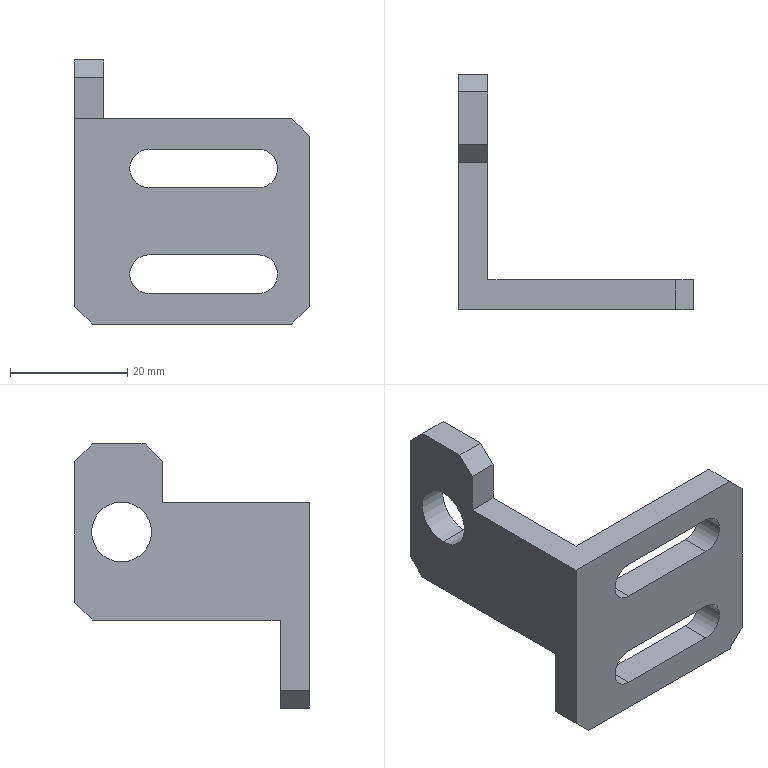Part | SolidWorks | features HoleWzd 2, ICE 2, Chamfer 1, Extrusion 1 | 1 solid | 27 faces | box 40 x 40 x 45 mm | volume 9137 mm3 | plane 21 | cylinder 6 | commonest cylinder face diameters 6.6 x4 10.2 x2
STEP:
#1=CARTESIAN_POINT('',(0.,-8.,35.1));
#2=VERTEX_POINT('',#1);
#3=CARTESIAN_POINT('',(0.,-8.,24.9));
#4=VERTEX_POINT('',#3);
#5=CARTESIAN_POINT('',(0.,-8.,30.));
#6=DIRECTION('',(1.,0.,0.));
#7=DIRECTION('',(0.,0.,-1.));
#8=AXIS2_PLACEMENT_3D('',#5,#6,#7);
#9=CIRCLE('',#8,5.1);
#10=EDGE_CURVE('',#2,#4,#9,.T.);
#11=ORIENTED_EDGE('',*,*,#10,.F.);
#12=CARTESIAN_POINT('',(5.,-8.,35.1));
#13=VERTEX_POINT('',#12);
#14=CARTESIAN_POINT('',(5.,-8.,35.1));
#15=DIRECTION('',(1.,0.,0.));
#16=VECTOR('',#15,1000.);
#17=LINE('',#14,#16);
#18=EDGE_CURVE('',#2,#13,#17,.T.);
#19=ORIENTED_EDGE('',*,*,#18,.T.);
#20=CARTESIAN_POINT('',(5.,-8.,24.9));
#21=VERTEX_POINT('',#20);
#22=CARTESIAN_POINT('',(5.,-8.,30.));
#23=DIRECTION('',(1.,0.,0.));
#24=DIRECTION('',(0.,0.,-1.));
#25=AXIS2_PLACEMENT_3D('',#22,#23,#24);
#26=CIRCLE('',#25,5.1);
#27=EDGE_CURVE('',#13,#21,#26,.T.);
#28=ORIENTED_EDGE('',*,*,#27,.T.);
#29=CARTESIAN_POINT('',(5.,-8.,24.9));
#30=DIRECTION('',(1.,0.,0.));
#31=VECTOR('',#30,1000.);
#32=LINE('',#29,#31);
#33=EDGE_CURVE('',#4,#21,#32,.T.);
#34=ORIENTED_EDGE('',*,*,#33,.F.);
#35=EDGE_LOOP('',(#11,#19,#28,#34));
#36=FACE_OUTER_BOUND('',#35,.T.);
#37=CARTESIAN_POINT('',(5.,-8.,30.));
#38=DIRECTION('',(1.,0.,0.));
#39=DIRECTION('',(0.,0.,-1.));
#40=AXIS2_PLACEMENT_3D('',#37,#38,#39);
#41=CYLINDRICAL_SURFACE('',#40,5.1);
#42=ADVANCED_FACE('',(#36),#41,.F.);
#43=CARTESIAN_POINT('',(12.7,-35.,5.2));
#44=VERTEX_POINT('',#43);
#45=CARTESIAN_POINT('',(12.7,-35.,11.8));
#46=VERTEX_POINT('',#45);
#47=CARTESIAN_POINT('',(12.7,-35.,8.5));
#48=DIRECTION('',(0.,1.,0.));
#49=DIRECTION('',(0.,0.,1.));
#50=AXIS2_PLACEMENT_3D('',#47,#48,#49);
#51=CIRCLE('',#50,3.3);
#52=EDGE_CURVE('',#44,#46,#51,.T.);
#53=ORIENTED_EDGE('',*,*,#52,.F.);
#54=CARTESIAN_POINT('',(31.3,-35.,5.2));
#55=VERTEX_POINT('',#54);
#56=CARTESIAN_POINT('',(12.7,-35.,5.2));
#57=DIRECTION('',(1.,0.,0.));
#58=VECTOR('',#57,1000.);
#59=LINE('',#56,#58);
#60=EDGE_CURVE('',#44,#55,#59,.T.);
#61=ORIENTED_EDGE('',*,*,#60,.T.);
#62=CARTESIAN_POINT('',(31.3,-35.,11.8));
#63=VERTEX_POINT('',#62);
#64=CARTESIAN_POINT('',(31.3,-35.,8.5));
#65=DIRECTION('',(0.,1.,0.));
#66=DIRECTION('',(0.,0.,1.));
#67=AXIS2_PLACEMENT_3D('',#64,#65,#66);
#68=CIRCLE('',#67,3.3);
#69=EDGE_CURVE('',#63,#55,#68,.T.);
#70=ORIENTED_EDGE('',*,*,#69,.F.);
#71=CARTESIAN_POINT('',(12.7,-35.,11.8));
#72=DIRECTION('',(1.,0.,0.));
#73=VECTOR('',#72,1000.);
#74=LINE('',#71,#73);
#75=EDGE_CURVE('',#46,#63,#74,.T.);
#76=ORIENTED_EDGE('',*,*,#75,.F.);
#77=EDGE_LOOP('',(#53,#61,#70,#76));
#78=FACE_BOUND('',#77,.T.);
#79=CARTESIAN_POINT('',(5.,-35.,35.));
#80=VERTEX_POINT('',#79);
#81=CARTESIAN_POINT('',(37.,-35.,35.));
#82=VERTEX_POINT('',#81);
#83=CARTESIAN_POINT('',(5.,-35.,35.));
#84=DIRECTION('',(1.,0.,0.));
#85=VECTOR('',#84,1000.);
#86=LINE('',#83,#85);
#87=EDGE_CURVE('',#80,#82,#86,.T.);
#88=ORIENTED_EDGE('',*,*,#87,.T.);
#89=CARTESIAN_POINT('',(40.,-35.,32.));
#90=VERTEX_POINT('',#89);
#91=CARTESIAN_POINT('',(40.,-35.,32.));
#92=DIRECTION('',(0.7071,0.,-0.7071));
#93=VECTOR('',#92,1000.);
#94=LINE('',#91,#93);
#95=EDGE_CURVE('',#82,#90,#94,.T.);
#96=ORIENTED_EDGE('',*,*,#95,.T.);
#97=CARTESIAN_POINT('',(40.,-35.,3.));
#98=VERTEX_POINT('',#97);
#99=CARTESIAN_POINT('',(40.,-35.,45.));
#100=DIRECTION('',(0.,0.,-1.));
#101=VECTOR('',#100,1000.);
#102=LINE('',#99,#101);
#103=EDGE_CURVE('',#90,#98,#102,.T.);
#104=ORIENTED_EDGE('',*,*,#103,.T.);
#105=CARTESIAN_POINT('',(37.,-35.,0.));
#106=VERTEX_POINT('',#105);
#107=CARTESIAN_POINT('',(40.,-35.,3.));
#108=DIRECTION('',(-0.7071,0.,-0.7071));
#109=VECTOR('',#108,1000.);
#110=LINE('',#107,#109);
#111=EDGE_CURVE('',#98,#106,#110,.T.);
#112=ORIENTED_EDGE('',*,*,#111,.T.);
#113=CARTESIAN_POINT('',(3.,-35.,0.));
#114=VERTEX_POINT('',#113);
#115=CARTESIAN_POINT('',(5.,-35.,0.));
#116=DIRECTION('',(-1.,0.,0.));
#117=VECTOR('',#116,1000.);
#118=LINE('',#115,#117);
#119=EDGE_CURVE('',#106,#114,#118,.T.);
#120=ORIENTED_EDGE('',*,*,#119,.T.);
#121=CARTESIAN_POINT('',(0.,-35.,3.));
#122=VERTEX_POINT('',#121);
#123=CARTESIAN_POINT('',(0.,-35.,3.));
#124=DIRECTION('',(-0.7071,0.,0.7071));
#125=VECTOR('',#124,1000.);
#126=LINE('',#123,#125);
#127=EDGE_CURVE('',#114,#122,#126,.T.);
#128=ORIENTED_EDGE('',*,*,#127,.T.);
#129=CARTESIAN_POINT('',(0.,-35.,15.));
#130=VERTEX_POINT('',#129);
#131=CARTESIAN_POINT('',(0.,-35.,0.));
#132=DIRECTION('',(0.,0.,1.));
#133=VECTOR('',#132,1000.);
#134=LINE('',#131,#133);
#135=EDGE_CURVE('',#122,#130,#134,.T.);
#136=ORIENTED_EDGE('',*,*,#135,.T.);
#137=CARTESIAN_POINT('',(5.,-35.,15.));
#138=VERTEX_POINT('',#137);
#139=CARTESIAN_POINT('',(5.,-35.,15.));
#140=DIRECTION('',(-1.,0.,0.));
#141=VECTOR('',#140,1000.);
#142=LINE('',#139,#141);
#143=EDGE_CURVE('',#138,#130,#142,.T.);
#144=ORIENTED_EDGE('',*,*,#143,.F.);
#145=CARTESIAN_POINT('',(5.,-35.,45.));
#146=DIRECTION('',(0.,0.,-1.));
#147=VECTOR('',#146,1000.);
#148=LINE('',#145,#147);
#149=EDGE_CURVE('',#80,#138,#148,.T.);
#150=ORIENTED_EDGE('',*,*,#149,.F.);
#151=EDGE_LOOP('',(#88,#96,#104,#112,#120,#128,#136,#144,#150));
#152=FACE_OUTER_BOUND('',#151,.T.);
#153=CARTESIAN_POINT('',(31.3,-35.,29.8));
#154=VERTEX_POINT('',#153);
#155=CARTESIAN_POINT('',(31.3,-35.,23.2));
#156=VERTEX_POINT('',#155);
#157=CARTESIAN_POINT('',(31.3,-35.,26.5));
#158=DIRECTION('',(0.,1.,0.));
#159=DIRECTION('',(0.,0.,1.));
#160=AXIS2_PLACEMENT_3D('',#157,#158,#159);
#161=CIRCLE('',#160,3.3);
#162=EDGE_CURVE('',#154,#156,#161,.T.);
#163=ORIENTED_EDGE('',*,*,#162,.F.);
#164=CARTESIAN_POINT('',(12.7,-35.,29.8));
#165=VERTEX_POINT('',#164);
#166=CARTESIAN_POINT('',(12.7,-35.,29.8));
#167=DIRECTION('',(1.,0.,0.));
#168=VECTOR('',#167,1000.);
#169=LINE('',#166,#168);
#170=EDGE_CURVE('',#165,#154,#169,.T.);
#171=ORIENTED_EDGE('',*,*,#170,.F.);
#172=CARTESIAN_POINT('',(12.7,-35.,23.2));
#173=VERTEX_POINT('',#172);
#174=CARTESIAN_POINT('',(12.7,-35.,26.5));
#175=DIRECTION('',(0.,1.,0.));
#176=DIRECTION('',(0.,0.,1.));
#177=AXIS2_PLACEMENT_3D('',#174,#175,#176);
#178=CIRCLE('',#177,3.3);
#179=EDGE_CURVE('',#173,#165,#178,.T.);
#180=ORIENTED_EDGE('',*,*,#179,.F.);
#181=CARTESIAN_POINT('',(12.7,-35.,23.2));
#182=DIRECTION('',(1.,0.,0.));
#183=VECTOR('',#182,1000.);
#184=LINE('',#181,#183);
#185=EDGE_CURVE('',#173,#156,#184,.T.);
#186=ORIENTED_EDGE('',*,*,#185,.T.);
#187=EDGE_LOOP('',(#163,#171,#180,#186));
#188=FACE_BOUND('',#187,.T.);
#189=CARTESIAN_POINT('',(5.,-35.,45.));
#190=DIRECTION('',(0.,-1.,0.));
#191=DIRECTION('',(0.,0.,-1.));
#192=AXIS2_PLACEMENT_3D('',#189,#190,#191);
#193=PLANE('',#192);
#194=ADVANCED_FACE('',(#78,#152,#188),#193,.F.);
#195=CARTESIAN_POINT('',(0.,-8.,30.));
#196=DIRECTION('',(1.,0.,0.));
#197=DIRECTION('',(0.,0.,-1.));
#198=AXIS2_PLACEMENT_3D('',#195,#196,#197);
#199=CIRCLE('',#198,5.1);
#200=EDGE_CURVE('',#4,#2,#199,.T.);
#201=ORIENTED_EDGE('',*,*,#200,.T.);
#202=ORIENTED_EDGE('',*,*,#10,.T.);
#203=EDGE_LOOP('',(#201,#202));
#204=FACE_BOUND('',#203,.T.);
#205=ORIENTED_EDGE('',*,*,#135,.F.);
#206=CARTESIAN_POINT('',(0.,-40.,3.));
#207=VERTEX_POINT('',#206);
#208=CARTESIAN_POINT('',(0.,-40.,3.));
#209=DIRECTION('',(0.,-1.,0.));
#210=VECTOR('',#209,1000.);
#211=LINE('',#208,#210);
#212=EDGE_CURVE('',#122,#207,#211,.T.);
#213=ORIENTED_EDGE('',*,*,#212,.T.);
#214=CARTESIAN_POINT('',(0.,-40.,35.));
#215=VERTEX_POINT('',#214);
#216=CARTESIAN_POINT('',(0.,-40.,45.));
#217=DIRECTION('',(0.,0.,-1.));
#218=VECTOR('',#217,1000.);
#219=LINE('',#216,#218);
#220=EDGE_CURVE('',#215,#207,#219,.T.);
#221=ORIENTED_EDGE('',*,*,#220,.F.);
#222=CARTESIAN_POINT('',(0.,-15.,35.));
#223=VERTEX_POINT('',#222);
#224=CARTESIAN_POINT('',(0.,-40.,35.));
#225=DIRECTION('',(0.,-1.,0.));
#226=VECTOR('',#225,1000.);
#227=LINE('',#224,#226);
#228=EDGE_CURVE('',#223,#215,#227,.T.);
#229=ORIENTED_EDGE('',*,*,#228,.F.);
#230=CARTESIAN_POINT('',(0.,-15.,42.));
#231=VERTEX_POINT('',#230);
#232=CARTESIAN_POINT('',(0.,-15.,45.));
#233=DIRECTION('',(0.,0.,-1.));
#234=VECTOR('',#233,1000.);
#235=LINE('',#232,#234);
#236=EDGE_CURVE('',#231,#223,#235,.T.);
#237=ORIENTED_EDGE('',*,*,#236,.F.);
#238=CARTESIAN_POINT('',(0.,-12.,45.));
#239=VERTEX_POINT('',#238);
#240=CARTESIAN_POINT('',(0.,-15.,42.));
#241=DIRECTION('',(0.,0.7071,0.7071));
#242=VECTOR('',#241,1000.);
#243=LINE('',#240,#242);
#244=EDGE_CURVE('',#231,#239,#243,.T.);
#245=ORIENTED_EDGE('',*,*,#244,.T.);
#246=CARTESIAN_POINT('',(0.,-3.,45.));
#247=VERTEX_POINT('',#246);
#248=CARTESIAN_POINT('',(0.,-40.,45.));
#249=DIRECTION('',(0.,-1.,0.));
#250=VECTOR('',#249,1000.);
#251=LINE('',#248,#250);
#252=EDGE_CURVE('',#247,#239,#251,.T.);
#253=ORIENTED_EDGE('',*,*,#252,.F.);
#254=CARTESIAN_POINT('',(0.,0.,42.));
#255=VERTEX_POINT('',#254);
#256=CARTESIAN_POINT('',(0.,-3.,45.));
#257=DIRECTION('',(0.,0.7071,-0.7071));
#258=VECTOR('',#257,1000.);
#259=LINE('',#256,#258);
#260=EDGE_CURVE('',#247,#255,#259,.T.);
#261=ORIENTED_EDGE('',*,*,#260,.T.);
#262=CARTESIAN_POINT('',(0.,0.,18.));
#263=VERTEX_POINT('',#262);
#264=CARTESIAN_POINT('',(0.,0.,45.));
#265=DIRECTION('',(0.,0.,-1.));
#266=VECTOR('',#265,1000.);
#267=LINE('',#264,#266);
#268=EDGE_CURVE('',#255,#263,#267,.T.);
#269=ORIENTED_EDGE('',*,*,#268,.T.);
#270=CARTESIAN_POINT('',(0.,-3.,15.));
#271=VERTEX_POINT('',#270);
#272=CARTESIAN_POINT('',(0.,0.,18.));
#273=DIRECTION('',(0.,-0.7071,-0.7071));
#274=VECTOR('',#273,1000.);
#275=LINE('',#272,#274);
#276=EDGE_CURVE('',#263,#271,#275,.T.);
#277=ORIENTED_EDGE('',*,*,#276,.T.);
#278=CARTESIAN_POINT('',(0.,0.,15.));
#279=DIRECTION('',(0.,1.,0.));
#280=VECTOR('',#279,1000.);
#281=LINE('',#278,#280);
#282=EDGE_CURVE('',#130,#271,#281,.T.);
#283=ORIENTED_EDGE('',*,*,#282,.F.);
#284=EDGE_LOOP('',(#205,#213,#221,#229,#237,#245,#253,#261,#269,#277,#283));
#285=FACE_OUTER_BOUND('',#284,.T.);
#286=CARTESIAN_POINT('',(0.,-40.,45.));
#287=DIRECTION('',(1.,0.,0.));
#288=DIRECTION('',(0.,0.,-1.));
#289=AXIS2_PLACEMENT_3D('',#286,#287,#288);
#290=PLANE('',#289);
#291=ADVANCED_FACE('',(#204,#285),#290,.F.);
#292=CARTESIAN_POINT('',(31.3,-40.,11.8));
#293=VERTEX_POINT('',#292);
#294=CARTESIAN_POINT('',(31.3,-40.,5.2));
#295=VERTEX_POINT('',#294);
#296=CARTESIAN_POINT('',(31.3,-40.,8.5));
#297=DIRECTION('',(0.,1.,0.));
#298=DIRECTION('',(-1.,0.,0.));
#299=AXIS2_PLACEMENT_3D('',#296,#297,#298);
#300=CIRCLE('',#299,3.3);
#301=EDGE_CURVE('',#293,#295,#300,.T.);
#302=ORIENTED_EDGE('',*,*,#301,.T.);
#303=CARTESIAN_POINT('',(12.7,-40.,5.2));
#304=VERTEX_POINT('',#303);
#305=CARTESIAN_POINT('',(40.,-40.,5.2));
#306=DIRECTION('',(-1.,0.,0.));
#307=VECTOR('',#306,1000.);
#308=LINE('',#305,#307);
#309=EDGE_CURVE('',#295,#304,#308,.T.);
#310=ORIENTED_EDGE('',*,*,#309,.T.);
#311=CARTESIAN_POINT('',(12.7,-40.,11.8));
#312=VERTEX_POINT('',#311);
#313=CARTESIAN_POINT('',(12.7,-40.,8.5));
#314=DIRECTION('',(0.,1.,0.));
#315=DIRECTION('',(-1.,0.,0.));
#316=AXIS2_PLACEMENT_3D('',#313,#314,#315);
#317=CIRCLE('',#316,3.3);
#318=EDGE_CURVE('',#304,#312,#317,.T.);
#319=ORIENTED_EDGE('',*,*,#318,.T.);
#320=CARTESIAN_POINT('',(40.,-40.,11.8));
#321=DIRECTION('',(1.,0.,0.));
#322=VECTOR('',#321,1000.);
#323=LINE('',#320,#322);
#324=EDGE_CURVE('',#312,#293,#323,.T.);
#325=ORIENTED_EDGE('',*,*,#324,.T.);
#326=EDGE_LOOP('',(#302,#310,#319,#325));
#327=FACE_BOUND('',#326,.T.);
#328=CARTESIAN_POINT('',(12.7,-40.,29.8));
#329=VERTEX_POINT('',#328);
#330=CARTESIAN_POINT('',(31.3,-40.,29.8));
#331=VERTEX_POINT('',#330);
#332=CARTESIAN_POINT('',(40.,-40.,29.8));
#333=DIRECTION('',(1.,0.,0.));
#334=VECTOR('',#333,1000.);
#335=LINE('',#332,#334);
#336=EDGE_CURVE('',#329,#331,#335,.T.);
#337=ORIENTED_EDGE('',*,*,#336,.T.);
#338=CARTESIAN_POINT('',(31.3,-40.,23.2));
#339=VERTEX_POINT('',#338);
#340=CARTESIAN_POINT('',(31.3,-40.,26.5));
#341=DIRECTION('',(0.,1.,0.));
#342=DIRECTION('',(-1.,0.,0.));
#343=AXIS2_PLACEMENT_3D('',#340,#341,#342);
#344=CIRCLE('',#343,3.3);
#345=EDGE_CURVE('',#331,#339,#344,.T.);
#346=ORIENTED_EDGE('',*,*,#345,.T.);
#347=CARTESIAN_POINT('',(12.7,-40.,23.2));
#348=VERTEX_POINT('',#347);
#349=CARTESIAN_POINT('',(40.,-40.,23.2));
#350=DIRECTION('',(-1.,0.,0.));
#351=VECTOR('',#350,1000.);
#352=LINE('',#349,#351);
#353=EDGE_CURVE('',#339,#348,#352,.T.);
#354=ORIENTED_EDGE('',*,*,#353,.T.);
#355=CARTESIAN_POINT('',(12.7,-40.,26.5));
#356=DIRECTION('',(0.,1.,0.));
#357=DIRECTION('',(-1.,0.,0.));
#358=AXIS2_PLACEMENT_3D('',#355,#356,#357);
#359=CIRCLE('',#358,3.3);
#360=EDGE_CURVE('',#348,#329,#359,.T.);
#361=ORIENTED_EDGE('',*,*,#360,.T.);
#362=EDGE_LOOP('',(#337,#346,#354,#361));
#363=FACE_BOUND('',#362,.T.);
#364=CARTESIAN_POINT('',(40.,-40.,32.));
#365=VERTEX_POINT('',#364);
#366=CARTESIAN_POINT('',(40.,-40.,3.));
#367=VERTEX_POINT('',#366);
#368=CARTESIAN_POINT('',(40.,-40.,45.));
#369=DIRECTION('',(0.,0.,-1.));
#370=VECTOR('',#369,1000.);
#371=LINE('',#368,#370);
#372=EDGE_CURVE('',#365,#367,#371,.T.);
#373=ORIENTED_EDGE('',*,*,#372,.F.);
#374=CARTESIAN_POINT('',(37.,-40.,35.));
#375=VERTEX_POINT('',#374);
#376=CARTESIAN_POINT('',(40.,-40.,32.));
#377=DIRECTION('',(-0.7071,0.,0.7071));
#378=VECTOR('',#377,1000.);
#379=LINE('',#376,#378);
#380=EDGE_CURVE('',#365,#375,#379,.T.);
#381=ORIENTED_EDGE('',*,*,#380,.T.);
#382=CARTESIAN_POINT('',(5.,-40.,35.));
#383=DIRECTION('',(-1.,0.,0.));
#384=VECTOR('',#383,1000.);
#385=LINE('',#382,#384);
#386=EDGE_CURVE('',#375,#215,#385,.T.);
#387=ORIENTED_EDGE('',*,*,#386,.T.);
#388=ORIENTED_EDGE('',*,*,#220,.T.);
#389=CARTESIAN_POINT('',(3.,-40.,0.));
#390=VERTEX_POINT('',#389);
#391=CARTESIAN_POINT('',(0.,-40.,3.));
#392=DIRECTION('',(0.7071,0.,-0.7071));
#393=VECTOR('',#392,1000.);
#394=LINE('',#391,#393);
#395=EDGE_CURVE('',#207,#390,#394,.T.);
#396=ORIENTED_EDGE('',*,*,#395,.T.);
#397=CARTESIAN_POINT('',(37.,-40.,0.));
#398=VERTEX_POINT('',#397);
#399=CARTESIAN_POINT('',(40.,-40.,0.));
#400=DIRECTION('',(1.,0.,0.));
#401=VECTOR('',#400,1000.);
#402=LINE('',#399,#401);
#403=EDGE_CURVE('',#390,#398,#402,.T.);
#404=ORIENTED_EDGE('',*,*,#403,.T.);
#405=CARTESIAN_POINT('',(40.,-40.,3.));
#406=DIRECTION('',(0.7071,0.,0.7071));
#407=VECTOR('',#406,1000.);
#408=LINE('',#405,#407);
#409=EDGE_CURVE('',#398,#367,#408,.T.);
#410=ORIENTED_EDGE('',*,*,#409,.T.);
#411=EDGE_LOOP('',(#373,#381,#387,#388,#396,#404,#410));
#412=FACE_OUTER_BOUND('',#411,.T.);
#413=CARTESIAN_POINT('',(40.,-40.,45.));
#414=DIRECTION('',(0.,1.,0.));
#415=DIRECTION('',(-1.,0.,0.));
#416=AXIS2_PLACEMENT_3D('',#413,#414,#415);
#417=PLANE('',#416);
#418=ADVANCED_FACE('',(#327,#363,#412),#417,.F.);
#419=ORIENTED_EDGE('',*,*,#103,.F.);
#420=CARTESIAN_POINT('',(40.,-35.,32.));
#421=DIRECTION('',(0.,-1.,0.));
#422=VECTOR('',#421,1000.);
#423=LINE('',#420,#422);
#424=EDGE_CURVE('',#90,#365,#423,.T.);
#425=ORIENTED_EDGE('',*,*,#424,.T.);
#426=ORIENTED_EDGE('',*,*,#372,.T.);
#427=CARTESIAN_POINT('',(40.,-35.,3.));
#428=DIRECTION('',(0.,1.,0.));
#429=VECTOR('',#428,1000.);
#430=LINE('',#427,#429);
#431=EDGE_CURVE('',#367,#98,#430,.T.);
#432=ORIENTED_EDGE('',*,*,#431,.T.);
#433=EDGE_LOOP('',(#419,#425,#426,#432));
#434=FACE_OUTER_BOUND('',#433,.T.);
#435=CARTESIAN_POINT('',(40.,-35.,45.));
#436=DIRECTION('',(-1.,0.,0.));
#437=DIRECTION('',(0.,0.,1.));
#438=AXIS2_PLACEMENT_3D('',#435,#436,#437);
#439=PLANE('',#438);
#440=ADVANCED_FACE('',(#434),#439,.F.);
#441=CARTESIAN_POINT('',(5.,-8.,30.));
#442=DIRECTION('',(1.,0.,0.));
#443=DIRECTION('',(0.,0.,-1.));
#444=AXIS2_PLACEMENT_3D('',#441,#442,#443);
#445=CIRCLE('',#444,5.1);
#446=EDGE_CURVE('',#21,#13,#445,.T.);
#447=ORIENTED_EDGE('',*,*,#446,.F.);
#448=ORIENTED_EDGE('',*,*,#27,.F.);
#449=EDGE_LOOP('',(#447,#448));
#450=FACE_BOUND('',#449,.T.);
#451=CARTESIAN_POINT('',(5.,-3.,15.));
#452=VERTEX_POINT('',#451);
#453=CARTESIAN_POINT('',(5.,0.,15.));
#454=DIRECTION('',(0.,1.,0.));
#455=VECTOR('',#454,1000.);
#456=LINE('',#453,#455);
#457=EDGE_CURVE('',#138,#452,#456,.T.);
#458=ORIENTED_EDGE('',*,*,#457,.T.);
#459=CARTESIAN_POINT('',(5.,0.,18.));
#460=VERTEX_POINT('',#459);
#461=CARTESIAN_POINT('',(5.,0.,18.));
#462=DIRECTION('',(0.,0.7071,0.7071));
#463=VECTOR('',#462,1000.);
#464=LINE('',#461,#463);
#465=EDGE_CURVE('',#452,#460,#464,.T.);
#466=ORIENTED_EDGE('',*,*,#465,.T.);
#467=CARTESIAN_POINT('',(5.,0.,42.));
#468=VERTEX_POINT('',#467);
#469=CARTESIAN_POINT('',(5.,0.,45.));
#470=DIRECTION('',(0.,0.,-1.));
#471=VECTOR('',#470,1000.);
#472=LINE('',#469,#471);
#473=EDGE_CURVE('',#468,#460,#472,.T.);
#474=ORIENTED_EDGE('',*,*,#473,.F.);
#475=CARTESIAN_POINT('',(5.,-3.,45.));
#476=VERTEX_POINT('',#475);
#477=CARTESIAN_POINT('',(5.,-3.,45.));
#478=DIRECTION('',(0.,-0.7071,0.7071));
#479=VECTOR('',#478,1000.);
#480=LINE('',#477,#479);
#481=EDGE_CURVE('',#468,#476,#480,.T.);
#482=ORIENTED_EDGE('',*,*,#481,.T.);
#483=CARTESIAN_POINT('',(5.,-12.,45.));
#484=VERTEX_POINT('',#483);
#485=CARTESIAN_POINT('',(5.,0.,45.));
#486=DIRECTION('',(0.,1.,0.));
#487=VECTOR('',#486,1000.);
#488=LINE('',#485,#487);
#489=EDGE_CURVE('',#484,#476,#488,.T.);
#490=ORIENTED_EDGE('',*,*,#489,.F.);
#491=CARTESIAN_POINT('',(5.,-15.,42.));
#492=VERTEX_POINT('',#491);
#493=CARTESIAN_POINT('',(5.,-15.,42.));
#494=DIRECTION('',(0.,-0.7071,-0.7071));
#495=VECTOR('',#494,1000.);
#496=LINE('',#493,#495);
#497=EDGE_CURVE('',#484,#492,#496,.T.);
#498=ORIENTED_EDGE('',*,*,#497,.T.);
#499=CARTESIAN_POINT('',(5.,-15.,35.));
#500=VERTEX_POINT('',#499);
#501=CARTESIAN_POINT('',(5.,-15.,45.));
#502=DIRECTION('',(0.,0.,-1.));
#503=VECTOR('',#502,1000.);
#504=LINE('',#501,#503);
#505=EDGE_CURVE('',#492,#500,#504,.T.);
#506=ORIENTED_EDGE('',*,*,#505,.T.);
#507=CARTESIAN_POINT('',(5.,-40.,35.));
#508=DIRECTION('',(0.,-1.,0.));
#509=VECTOR('',#508,1000.);
#510=LINE('',#507,#509);
#511=EDGE_CURVE('',#500,#80,#510,.T.);
#512=ORIENTED_EDGE('',*,*,#511,.T.);
#513=ORIENTED_EDGE('',*,*,#149,.T.);
#514=EDGE_LOOP('',(#458,#466,#474,#482,#490,#498,#506,#512,#513));
#515=FACE_OUTER_BOUND('',#514,.T.);
#516=CARTESIAN_POINT('',(5.,0.,45.));
#517=DIRECTION('',(-1.,0.,0.));
#518=DIRECTION('',(0.,-1.,0.));
#519=AXIS2_PLACEMENT_3D('',#516,#517,#518);
#520=PLANE('',#519);
#521=ADVANCED_FACE('',(#450,#515),#520,.F.);
#522=ORIENTED_EDGE('',*,*,#473,.T.);
#523=CARTESIAN_POINT('',(0.,0.,18.));
#524=DIRECTION('',(-1.,0.,0.));
#525=VECTOR('',#524,1000.);
#526=LINE('',#523,#525);
#527=EDGE_CURVE('',#460,#263,#526,.T.);
#528=ORIENTED_EDGE('',*,*,#527,.T.);
#529=ORIENTED_EDGE('',*,*,#268,.F.);
#530=CARTESIAN_POINT('',(0.,0.,42.));
#531=DIRECTION('',(1.,0.,0.));
#532=VECTOR('',#531,1000.);
#533=LINE('',#530,#532);
#534=EDGE_CURVE('',#255,#468,#533,.T.);
#535=ORIENTED_EDGE('',*,*,#534,.T.);
#536=EDGE_LOOP('',(#522,#528,#529,#535));
#537=FACE_OUTER_BOUND('',#536,.T.);
#538=CARTESIAN_POINT('',(0.,0.,45.));
#539=DIRECTION('',(0.,-1.,0.));
#540=DIRECTION('',(0.,0.,-1.));
#541=AXIS2_PLACEMENT_3D('',#538,#539,#540);
#542=PLANE('',#541);
#543=ADVANCED_FACE('',(#537),#542,.F.);
#544=ORIENTED_EDGE('',*,*,#252,.T.);
#545=CARTESIAN_POINT('',(0.,-12.,45.));
#546=DIRECTION('',(1.,0.,0.));
#547=VECTOR('',#546,1000.);
#548=LINE('',#545,#547);
#549=EDGE_CURVE('',#239,#484,#548,.T.);
#550=ORIENTED_EDGE('',*,*,#549,.T.);
#551=ORIENTED_EDGE('',*,*,#489,.T.);
#552=CARTESIAN_POINT('',(0.,-3.,45.));
#553=DIRECTION('',(-1.,0.,0.));
#554=VECTOR('',#553,1000.);
#555=LINE('',#552,#554);
#556=EDGE_CURVE('',#476,#247,#555,.T.);
#557=ORIENTED_EDGE('',*,*,#556,.T.);
#558=EDGE_LOOP('',(#544,#550,#551,#557));
#559=FACE_OUTER_BOUND('',#558,.T.);
#560=CARTESIAN_POINT('',(0.,0.,45.));
#561=DIRECTION('',(0.,0.,-1.));
#562=DIRECTION('',(-1.,0.,0.));
#563=AXIS2_PLACEMENT_3D('',#560,#561,#562);
#564=PLANE('',#563);
#565=ADVANCED_FACE('',(#559),#564,.F.);
#566=ORIENTED_EDGE('',*,*,#119,.F.);
#567=CARTESIAN_POINT('',(37.,-40.,0.));
#568=DIRECTION('',(0.,-1.,0.));
#569=VECTOR('',#568,1000.);
#570=LINE('',#567,#569);
#571=EDGE_CURVE('',#106,#398,#570,.T.);
#572=ORIENTED_EDGE('',*,*,#571,.T.);
#573=ORIENTED_EDGE('',*,*,#403,.F.);
#574=CARTESIAN_POINT('',(3.,-35.,0.));
#575=DIRECTION('',(0.,1.,0.));
#576=VECTOR('',#575,1000.);
#577=LINE('',#574,#576);
#578=EDGE_CURVE('',#390,#114,#577,.T.);
#579=ORIENTED_EDGE('',*,*,#578,.T.);
#580=EDGE_LOOP('',(#566,#572,#573,#579));
#581=FACE_OUTER_BOUND('',#580,.T.);
#582=CARTESIAN_POINT('',(0.,0.,0.));
#583=DIRECTION('',(0.,0.,-1.));
#584=DIRECTION('',(-1.,0.,0.));
#585=AXIS2_PLACEMENT_3D('',#582,#583,#584);
#586=PLANE('',#585);
#587=ADVANCED_FACE('',(#581),#586,.T.);
#588=ORIENTED_EDGE('',*,*,#282,.T.);
#589=CARTESIAN_POINT('',(5.,-3.,15.));
#590=DIRECTION('',(1.,0.,0.));
#591=VECTOR('',#590,1000.);
#592=LINE('',#589,#591);
#593=EDGE_CURVE('',#271,#452,#592,.T.);
#594=ORIENTED_EDGE('',*,*,#593,.T.);
#595=ORIENTED_EDGE('',*,*,#457,.F.);
#596=ORIENTED_EDGE('',*,*,#143,.T.);
#597=EDGE_LOOP('',(#588,#594,#595,#596));
#598=FACE_OUTER_BOUND('',#597,.T.);
#599=CARTESIAN_POINT('',(5.,0.,15.));
#600=DIRECTION('',(0.,0.,1.));
#601=DIRECTION('',(0.,-1.,0.));
#602=AXIS2_PLACEMENT_3D('',#599,#600,#601);
#603=PLANE('',#602);
#604=ADVANCED_FACE('',(#598),#603,.F.);
#605=ORIENTED_EDGE('',*,*,#386,.F.);
#606=CARTESIAN_POINT('',(37.,-40.,35.));
#607=DIRECTION('',(0.,1.,0.));
#608=VECTOR('',#607,1000.);
#609=LINE('',#606,#608);
#610=EDGE_CURVE('',#375,#82,#609,.T.);
#611=ORIENTED_EDGE('',*,*,#610,.T.);
#612=ORIENTED_EDGE('',*,*,#87,.F.);
#613=ORIENTED_EDGE('',*,*,#511,.F.);
#614=CARTESIAN_POINT('',(5.,-15.,35.));
#615=DIRECTION('',(-1.,0.,0.));
#616=VECTOR('',#615,1000.);
#617=LINE('',#614,#616);
#618=EDGE_CURVE('',#500,#223,#617,.T.);
#619=ORIENTED_EDGE('',*,*,#618,.T.);
#620=ORIENTED_EDGE('',*,*,#228,.T.);
#621=EDGE_LOOP('',(#605,#611,#612,#613,#619,#620));
#622=FACE_OUTER_BOUND('',#621,.T.);
#623=CARTESIAN_POINT('',(5.,-40.,35.));
#624=DIRECTION('',(0.,0.,-1.));
#625=DIRECTION('',(-1.,0.,0.));
#626=AXIS2_PLACEMENT_3D('',#623,#624,#625);
#627=PLANE('',#626);
#628=ADVANCED_FACE('',(#622),#627,.F.);
#629=ORIENTED_EDGE('',*,*,#505,.F.);
#630=CARTESIAN_POINT('',(5.,-15.,42.));
#631=DIRECTION('',(-1.,0.,0.));
#632=VECTOR('',#631,1000.);
#633=LINE('',#630,#632);
#634=EDGE_CURVE('',#492,#231,#633,.T.);
#635=ORIENTED_EDGE('',*,*,#634,.T.);
#636=ORIENTED_EDGE('',*,*,#236,.T.);
#637=ORIENTED_EDGE('',*,*,#618,.F.);
#638=EDGE_LOOP('',(#629,#635,#636,#637));
#639=FACE_OUTER_BOUND('',#638,.T.);
#640=CARTESIAN_POINT('',(5.,-15.,45.));
#641=DIRECTION('',(0.,1.,0.));
#642=DIRECTION('',(0.,0.,1.));
#643=AXIS2_PLACEMENT_3D('',#640,#641,#642);
#644=PLANE('',#643);
#645=ADVANCED_FACE('',(#639),#644,.F.);
#646=ORIENTED_EDGE('',*,*,#18,.F.);
#647=ORIENTED_EDGE('',*,*,#200,.F.);
#648=ORIENTED_EDGE('',*,*,#33,.T.);
#649=ORIENTED_EDGE('',*,*,#446,.T.);
#650=EDGE_LOOP('',(#646,#647,#648,#649));
#651=FACE_OUTER_BOUND('',#650,.T.);
#652=CARTESIAN_POINT('',(5.,-8.,30.));
#653=DIRECTION('',(1.,0.,0.));
#654=DIRECTION('',(0.,0.,-1.));
#655=AXIS2_PLACEMENT_3D('',#652,#653,#654);
#656=CYLINDRICAL_SURFACE('',#655,5.1);
#657=ADVANCED_FACE('',(#651),#656,.F.);
#658=ORIENTED_EDGE('',*,*,#95,.F.);
#659=ORIENTED_EDGE('',*,*,#610,.F.);
#660=ORIENTED_EDGE('',*,*,#380,.F.);
#661=ORIENTED_EDGE('',*,*,#424,.F.);
#662=EDGE_LOOP('',(#658,#659,#660,#661));
#663=FACE_OUTER_BOUND('',#662,.T.);
#664=CARTESIAN_POINT('',(40.,-35.,32.));
#665=DIRECTION('',(-0.7071,0.,-0.7071));
#666=DIRECTION('',(0.,-1.,0.));
#667=AXIS2_PLACEMENT_3D('',#664,#665,#666);
#668=PLANE('',#667);
#669=ADVANCED_FACE('',(#663),#668,.F.);
#670=ORIENTED_EDGE('',*,*,#409,.F.);
#671=ORIENTED_EDGE('',*,*,#571,.F.);
#672=ORIENTED_EDGE('',*,*,#111,.F.);
#673=ORIENTED_EDGE('',*,*,#431,.F.);
#674=EDGE_LOOP('',(#670,#671,#672,#673));
#675=FACE_OUTER_BOUND('',#674,.T.);
#676=CARTESIAN_POINT('',(40.,-35.,3.));
#677=DIRECTION('',(0.7071,0.,-0.7071));
#678=DIRECTION('',(0.,-1.,0.));
#679=AXIS2_PLACEMENT_3D('',#676,#677,#678);
#680=PLANE('',#679);
#681=ADVANCED_FACE('',(#675),#680,.T.);
#682=ORIENTED_EDGE('',*,*,#127,.F.);
#683=ORIENTED_EDGE('',*,*,#578,.F.);
#684=ORIENTED_EDGE('',*,*,#395,.F.);
#685=ORIENTED_EDGE('',*,*,#212,.F.);
#686=EDGE_LOOP('',(#682,#683,#684,#685));
#687=FACE_OUTER_BOUND('',#686,.T.);
#688=CARTESIAN_POINT('',(0.,-40.,3.));
#689=DIRECTION('',(-0.7071,0.,-0.7071));
#690=DIRECTION('',(0.,1.,0.));
#691=AXIS2_PLACEMENT_3D('',#688,#689,#690);
#692=PLANE('',#691);
#693=ADVANCED_FACE('',(#687),#692,.T.);
#694=ORIENTED_EDGE('',*,*,#465,.F.);
#695=ORIENTED_EDGE('',*,*,#593,.F.);
#696=ORIENTED_EDGE('',*,*,#276,.F.);
#697=ORIENTED_EDGE('',*,*,#527,.F.);
#698=EDGE_LOOP('',(#694,#695,#696,#697));
#699=FACE_OUTER_BOUND('',#698,.T.);
#700=CARTESIAN_POINT('',(0.,0.,18.));
#701=DIRECTION('',(0.,-0.7071,0.7071));
#702=DIRECTION('',(-1.,0.,0.));
#703=AXIS2_PLACEMENT_3D('',#700,#701,#702);
#704=PLANE('',#703);
#705=ADVANCED_FACE('',(#699),#704,.F.);
#706=ORIENTED_EDGE('',*,*,#497,.F.);
#707=ORIENTED_EDGE('',*,*,#549,.F.);
#708=ORIENTED_EDGE('',*,*,#244,.F.);
#709=ORIENTED_EDGE('',*,*,#634,.F.);
#710=EDGE_LOOP('',(#706,#707,#708,#709));
#711=FACE_OUTER_BOUND('',#710,.T.);
#712=CARTESIAN_POINT('',(5.,-15.,42.));
#713=DIRECTION('',(0.,0.7071,-0.7071));
#714=DIRECTION('',(-1.,0.,0.));
#715=AXIS2_PLACEMENT_3D('',#712,#713,#714);
#716=PLANE('',#715);
#717=ADVANCED_FACE('',(#711),#716,.F.);
#718=ORIENTED_EDGE('',*,*,#481,.F.);
#719=ORIENTED_EDGE('',*,*,#534,.F.);
#720=ORIENTED_EDGE('',*,*,#260,.F.);
#721=ORIENTED_EDGE('',*,*,#556,.F.);
#722=EDGE_LOOP('',(#718,#719,#720,#721));
#723=FACE_OUTER_BOUND('',#722,.T.);
#724=CARTESIAN_POINT('',(0.,-3.,45.));
#725=DIRECTION('',(0.,-0.7071,-0.7071));
#726=DIRECTION('',(-1.,0.,0.));
#727=AXIS2_PLACEMENT_3D('',#724,#725,#726);
#728=PLANE('',#727);
#729=ADVANCED_FACE('',(#723),#728,.F.);
#730=CARTESIAN_POINT('',(12.7,-35.,23.2));
#731=DIRECTION('',(0.,-1.,0.));
#732=VECTOR('',#731,1000.);
#733=LINE('',#730,#732);
#734=EDGE_CURVE('',#173,#348,#733,.T.);
#735=ORIENTED_EDGE('',*,*,#734,.F.);
#736=ORIENTED_EDGE('',*,*,#179,.T.);
#737=CARTESIAN_POINT('',(12.7,-35.,29.8));
#738=DIRECTION('',(0.,1.,0.));
#739=VECTOR('',#738,1000.);
#740=LINE('',#737,#739);
#741=EDGE_CURVE('',#329,#165,#740,.T.);
#742=ORIENTED_EDGE('',*,*,#741,.F.);
#743=ORIENTED_EDGE('',*,*,#360,.F.);
#744=EDGE_LOOP('',(#735,#736,#742,#743));
#745=FACE_OUTER_BOUND('',#744,.T.);
#746=CARTESIAN_POINT('',(12.7,-35.,26.5));
#747=DIRECTION('',(0.,1.,0.));
#748=DIRECTION('',(0.,0.,1.));
#749=AXIS2_PLACEMENT_3D('',#746,#747,#748);
#750=CYLINDRICAL_SURFACE('',#749,3.3);
#751=ADVANCED_FACE('',(#745),#750,.F.);
#752=CARTESIAN_POINT('',(31.3,-35.,29.8));
#753=DIRECTION('',(0.,-1.,0.));
#754=VECTOR('',#753,1000.);
#755=LINE('',#752,#754);
#756=EDGE_CURVE('',#154,#331,#755,.T.);
#757=ORIENTED_EDGE('',*,*,#756,.F.);
#758=ORIENTED_EDGE('',*,*,#162,.T.);
#759=CARTESIAN_POINT('',(31.3,-35.,23.2));
#760=DIRECTION('',(0.,1.,0.));
#761=VECTOR('',#760,1000.);
#762=LINE('',#759,#761);
#763=EDGE_CURVE('',#339,#156,#762,.T.);
#764=ORIENTED_EDGE('',*,*,#763,.F.);
#765=ORIENTED_EDGE('',*,*,#345,.F.);
#766=EDGE_LOOP('',(#757,#758,#764,#765));
#767=FACE_OUTER_BOUND('',#766,.T.);
#768=CARTESIAN_POINT('',(31.3,-35.,26.5));
#769=DIRECTION('',(0.,1.,0.));
#770=DIRECTION('',(0.,0.,1.));
#771=AXIS2_PLACEMENT_3D('',#768,#769,#770);
#772=CYLINDRICAL_SURFACE('',#771,3.3);
#773=ADVANCED_FACE('',(#767),#772,.F.);
#774=ORIENTED_EDGE('',*,*,#763,.T.);
#775=ORIENTED_EDGE('',*,*,#185,.F.);
#776=ORIENTED_EDGE('',*,*,#734,.T.);
#777=ORIENTED_EDGE('',*,*,#353,.F.);
#778=EDGE_LOOP('',(#774,#775,#776,#777));
#779=FACE_OUTER_BOUND('',#778,.T.);
#780=CARTESIAN_POINT('',(12.7,-35.,23.2));
#781=DIRECTION('',(0.,0.,-1.));
#782=DIRECTION('',(-1.,0.,0.));
#783=AXIS2_PLACEMENT_3D('',#780,#781,#782);
#784=PLANE('',#783);
#785=ADVANCED_FACE('',(#779),#784,.F.);
#786=ORIENTED_EDGE('',*,*,#741,.T.);
#787=ORIENTED_EDGE('',*,*,#170,.T.);
#788=ORIENTED_EDGE('',*,*,#756,.T.);
#789=ORIENTED_EDGE('',*,*,#336,.F.);
#790=EDGE_LOOP('',(#786,#787,#788,#789));
#791=FACE_OUTER_BOUND('',#790,.T.);
#792=CARTESIAN_POINT('',(12.7,-35.,29.8));
#793=DIRECTION('',(0.,0.,1.));
#794=DIRECTION('',(1.,0.,0.));
#795=AXIS2_PLACEMENT_3D('',#792,#793,#794);
#796=PLANE('',#795);
#797=ADVANCED_FACE('',(#791),#796,.F.);
#798=CARTESIAN_POINT('',(31.3,-35.,5.2));
#799=DIRECTION('',(0.,1.,0.));
#800=VECTOR('',#799,1000.);
#801=LINE('',#798,#800);
#802=EDGE_CURVE('',#295,#55,#801,.T.);
#803=ORIENTED_EDGE('',*,*,#802,.T.);
#804=ORIENTED_EDGE('',*,*,#60,.F.);
#805=CARTESIAN_POINT('',(12.7,-35.,5.2));
#806=DIRECTION('',(0.,-1.,0.));
#807=VECTOR('',#806,1000.);
#808=LINE('',#805,#807);
#809=EDGE_CURVE('',#44,#304,#808,.T.);
#810=ORIENTED_EDGE('',*,*,#809,.T.);
#811=ORIENTED_EDGE('',*,*,#309,.F.);
#812=EDGE_LOOP('',(#803,#804,#810,#811));
#813=FACE_OUTER_BOUND('',#812,.T.);
#814=CARTESIAN_POINT('',(12.7,-35.,5.2));
#815=DIRECTION('',(0.,0.,-1.));
#816=DIRECTION('',(-1.,0.,0.));
#817=AXIS2_PLACEMENT_3D('',#814,#815,#816);
#818=PLANE('',#817);
#819=ADVANCED_FACE('',(#813),#818,.F.);
#820=CARTESIAN_POINT('',(31.3,-35.,11.8));
#821=DIRECTION('',(0.,-1.,0.));
#822=VECTOR('',#821,1000.);
#823=LINE('',#820,#822);
#824=EDGE_CURVE('',#63,#293,#823,.T.);
#825=ORIENTED_EDGE('',*,*,#824,.F.);
#826=ORIENTED_EDGE('',*,*,#69,.T.);
#827=ORIENTED_EDGE('',*,*,#802,.F.);
#828=ORIENTED_EDGE('',*,*,#301,.F.);
#829=EDGE_LOOP('',(#825,#826,#827,#828));
#830=FACE_OUTER_BOUND('',#829,.T.);
#831=CARTESIAN_POINT('',(31.3,-35.,8.5));
#832=DIRECTION('',(0.,1.,0.));
#833=DIRECTION('',(0.,0.,1.));
#834=AXIS2_PLACEMENT_3D('',#831,#832,#833);
#835=CYLINDRICAL_SURFACE('',#834,3.3);
#836=ADVANCED_FACE('',(#830),#835,.F.);
#837=ORIENTED_EDGE('',*,*,#809,.F.);
#838=ORIENTED_EDGE('',*,*,#52,.T.);
#839=CARTESIAN_POINT('',(12.7,-35.,11.8));
#840=DIRECTION('',(0.,1.,0.));
#841=VECTOR('',#840,1000.);
#842=LINE('',#839,#841);
#843=EDGE_CURVE('',#312,#46,#842,.T.);
#844=ORIENTED_EDGE('',*,*,#843,.F.);
#845=ORIENTED_EDGE('',*,*,#318,.F.);
#846=EDGE_LOOP('',(#837,#838,#844,#845));
#847=FACE_OUTER_BOUND('',#846,.T.);
#848=CARTESIAN_POINT('',(12.7,-35.,8.5));
#849=DIRECTION('',(0.,1.,0.));
#850=DIRECTION('',(0.,0.,1.));
#851=AXIS2_PLACEMENT_3D('',#848,#849,#850);
#852=CYLINDRICAL_SURFACE('',#851,3.3);
#853=ADVANCED_FACE('',(#847),#852,.F.);
#854=ORIENTED_EDGE('',*,*,#843,.T.);
#855=ORIENTED_EDGE('',*,*,#75,.T.);
#856=ORIENTED_EDGE('',*,*,#824,.T.);
#857=ORIENTED_EDGE('',*,*,#324,.F.);
#858=EDGE_LOOP('',(#854,#855,#856,#857));
#859=FACE_OUTER_BOUND('',#858,.T.);
#860=CARTESIAN_POINT('',(12.7,-35.,11.8));
#861=DIRECTION('',(0.,0.,1.));
#862=DIRECTION('',(1.,0.,0.));
#863=AXIS2_PLACEMENT_3D('',#860,#861,#862);
#864=PLANE('',#863);
#865=ADVANCED_FACE('',(#859),#864,.F.);
#866=CLOSED_SHELL('',(#42,#194,#291,#418,#440,#521,#543,#565,#587,#604,#628,#645,#657,#669,#681,#693,#705,#717,#729,#751,#773,#785,#797,#819,#836,#853,#865));
#867=MANIFOLD_SOLID_BREP('',#866);
#868=CARTESIAN_POINT('',(0.,0.,0.));
#869=DIRECTION('',(0.,0.,1.));
#870=DIRECTION('',(1.,0.,0.));
#871=AXIS2_PLACEMENT_3D('',#868,#869,#870);
#872=(LENGTH_UNIT()NAMED_UNIT(*)SI_UNIT(.MILLI.,.METRE.));
#873=UNCERTAINTY_MEASURE_WITH_UNIT(LENGTH_MEASURE(0.00001),#872,'','');
#874=(NAMED_UNIT(*)PLANE_ANGLE_UNIT()SI_UNIT($,.RADIAN.));
#875=(NAMED_UNIT(*)SI_UNIT($,.STERADIAN.)SOLID_ANGLE_UNIT());
#876=(GEOMETRIC_REPRESENTATION_CONTEXT(3)GLOBAL_UNCERTAINTY_ASSIGNED_CONTEXT((#873))GLOBAL_UNIT_ASSIGNED_CONTEXT((#872,#874,#875))REPRESENTATION_CONTEXT('',''));
#877=ADVANCED_BREP_SHAPE_REPRESENTATION('',(#867,#871),#876);